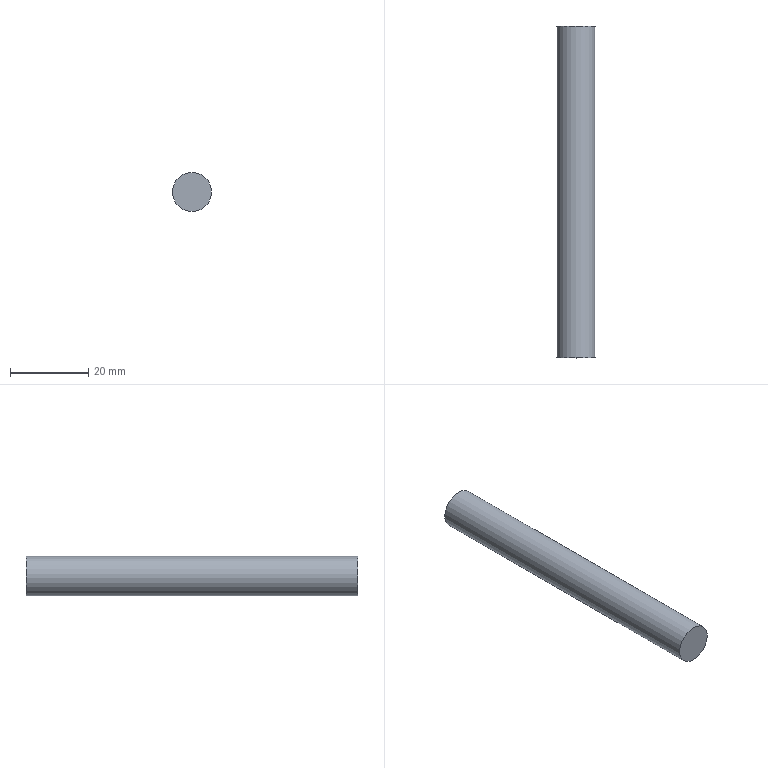Part | NX | features solid 2 | 1 solid | 3 faces | box 10 x 85 x 10 mm | volume 6676 mm3 | plane 2 | cylinder 1 | commonest cylinder face diameters 10 x1
STEP:
#1=CARTESIAN_POINT('',(-75.,417.,-37.));
#2=VERTEX_POINT('',#1);
#3=CARTESIAN_POINT('',(-75.,417.,-32.));
#4=DIRECTION('',(0.,-1.,0.));
#5=DIRECTION('',(0.,0.,-1.));
#6=AXIS2_PLACEMENT_3D('',#3,#4,#5);
#7=CIRCLE('',#6,5.);
#8=EDGE_CURVE('',#2,#2,#7,.T.);
#9=ORIENTED_EDGE('',*,*,#8,.T.);
#10=EDGE_LOOP('',(#9));
#11=FACE_BOUND('',#10,.T.);
#12=CARTESIAN_POINT('',(-75.,332.,-27.));
#13=VERTEX_POINT('',#12);
#14=CARTESIAN_POINT('',(-75.,332.,-32.));
#15=DIRECTION('',(0.,1.,0.));
#16=DIRECTION('',(0.,0.,1.));
#17=AXIS2_PLACEMENT_3D('',#14,#15,#16);
#18=CIRCLE('',#17,5.);
#19=EDGE_CURVE('',#13,#13,#18,.F.);
#20=ORIENTED_EDGE('',*,*,#19,.F.);
#21=EDGE_LOOP('',(#20));
#22=FACE_BOUND('',#21,.T.);
#23=CARTESIAN_POINT('',(-75.,377.,-32.));
#24=DIRECTION('',(0.,-1.,0.));
#25=DIRECTION('',(0.,0.,-1.));
#26=AXIS2_PLACEMENT_3D('',#23,#24,#25);
#27=CYLINDRICAL_SURFACE('',#26,5.);
#28=ADVANCED_FACE('',(#11,#22),#27,.T.);
#29=ORIENTED_EDGE('',*,*,#8,.F.);
#30=EDGE_LOOP('',(#29));
#31=FACE_BOUND('',#30,.T.);
#32=CARTESIAN_POINT('',(-85.,417.,27.));
#33=DIRECTION('',(0.,-1.,0.));
#34=DIRECTION('',(0.,0.,-1.));
#35=AXIS2_PLACEMENT_3D('',#32,#33,#34);
#36=PLANE('',#35);
#37=ADVANCED_FACE('',(#31),#36,.F.);
#38=ORIENTED_EDGE('',*,*,#19,.T.);
#39=EDGE_LOOP('',(#38));
#40=FACE_BOUND('',#39,.T.);
#41=CARTESIAN_POINT('',(-75.,332.,-32.));
#42=DIRECTION('',(0.,1.,0.));
#43=DIRECTION('',(0.,0.,1.));
#44=AXIS2_PLACEMENT_3D('',#41,#42,#43);
#45=PLANE('',#44);
#46=ADVANCED_FACE('',(#40),#45,.F.);
#47=CLOSED_SHELL('',(#28,#37,#46));
#48=MANIFOLD_SOLID_BREP('',#47);
#49=(LENGTH_UNIT()NAMED_UNIT(*)SI_UNIT(.MILLI.,.METRE.));
#50=UNCERTAINTY_MEASURE_WITH_UNIT(LENGTH_MEASURE(0.00001),#49,'','');
#51=(NAMED_UNIT(*)PLANE_ANGLE_UNIT()SI_UNIT($,.RADIAN.));
#52=(NAMED_UNIT(*)SI_UNIT($,.STERADIAN.)SOLID_ANGLE_UNIT());
#53=(GEOMETRIC_REPRESENTATION_CONTEXT(3)GLOBAL_UNCERTAINTY_ASSIGNED_CONTEXT((#50))GLOBAL_UNIT_ASSIGNED_CONTEXT((#49,#51,#52))REPRESENTATION_CONTEXT('',''));
#54=ADVANCED_BREP_SHAPE_REPRESENTATION('',(#48),#53);